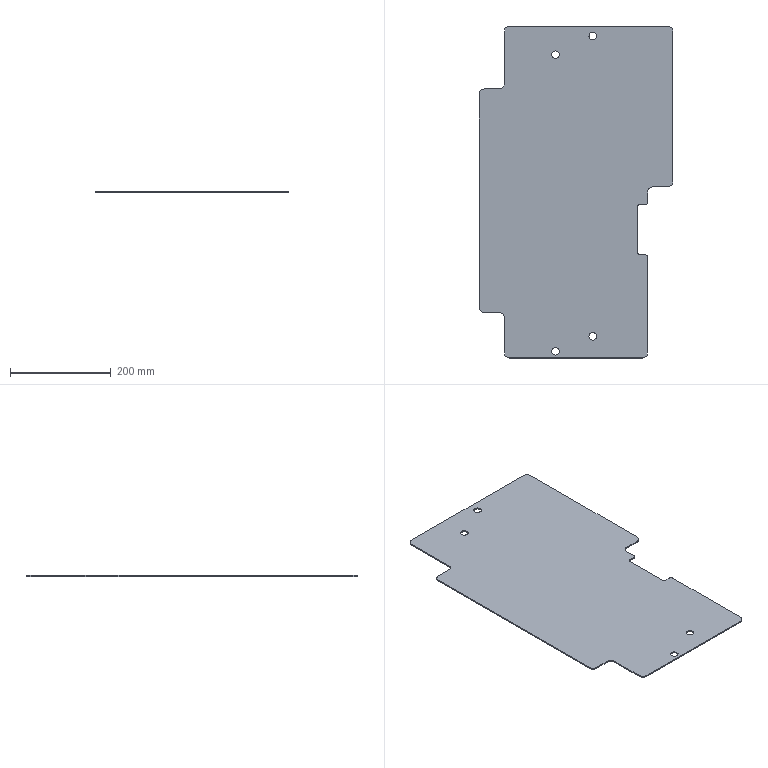Part | SolidWorks | features FlatPattern 1, SMBaseFlange 1, SheetMetal 1 | 1 solid | 38 faces | box 384.5 x 660 x 2.3 mm | volume 513423 mm3 | cylinder 22 | plane 16 | commonest cylinder face diameters 20 x10 15 x8 10 x4
STEP:
#1=CARTESIAN_POINT('',(163.,-881.,2.3));
#2=VERTEX_POINT('',#1);
#3=CARTESIAN_POINT('',(178.,-881.,2.3));
#4=VERTEX_POINT('',#3);
#5=CARTESIAN_POINT('',(170.5,-881.,2.3));
#6=DIRECTION('',(0.,0.,1.));
#7=DIRECTION('',(1.,0.,0.));
#8=AXIS2_PLACEMENT_3D('',#5,#6,#7);
#9=CIRCLE('',#8,7.5);
#10=EDGE_CURVE('',#2,#4,#9,.T.);
#11=ORIENTED_EDGE('',*,*,#10,.T.);
#12=CARTESIAN_POINT('',(178.,-881.,0.));
#13=VERTEX_POINT('',#12);
#14=CARTESIAN_POINT('',(178.,-881.,2.3));
#15=DIRECTION('',(0.,0.,-1.));
#16=VECTOR('',#15,1000.);
#17=LINE('',#14,#16);
#18=EDGE_CURVE('',#4,#13,#17,.T.);
#19=ORIENTED_EDGE('',*,*,#18,.T.);
#20=CARTESIAN_POINT('',(163.,-881.,0.));
#21=VERTEX_POINT('',#20);
#22=CARTESIAN_POINT('',(170.5,-881.,0.));
#23=DIRECTION('',(0.,0.,1.));
#24=DIRECTION('',(1.,0.,0.));
#25=AXIS2_PLACEMENT_3D('',#22,#23,#24);
#26=CIRCLE('',#25,7.5);
#27=EDGE_CURVE('',#21,#13,#26,.T.);
#28=ORIENTED_EDGE('',*,*,#27,.F.);
#29=CARTESIAN_POINT('',(163.,-881.,2.3));
#30=DIRECTION('',(0.,0.,-1.));
#31=VECTOR('',#30,1000.);
#32=LINE('',#29,#31);
#33=EDGE_CURVE('',#2,#21,#32,.T.);
#34=ORIENTED_EDGE('',*,*,#33,.F.);
#35=EDGE_LOOP('',(#11,#19,#28,#34));
#36=FACE_OUTER_BOUND('',#35,.T.);
#37=CARTESIAN_POINT('',(170.5,-881.,2.3));
#38=DIRECTION('',(0.,0.,-1.));
#39=DIRECTION('',(-1.,0.,0.));
#40=AXIS2_PLACEMENT_3D('',#37,#38,#39);
#41=CYLINDRICAL_SURFACE('',#40,7.5);
#42=ADVANCED_FACE('',(#36),#41,.F.);
#43=CARTESIAN_POINT('',(237.,-851.,2.3));
#44=VERTEX_POINT('',#43);
#45=CARTESIAN_POINT('',(252.,-851.,2.3));
#46=VERTEX_POINT('',#45);
#47=CARTESIAN_POINT('',(244.5,-851.,2.3));
#48=DIRECTION('',(0.,0.,1.));
#49=DIRECTION('',(1.,0.,0.));
#50=AXIS2_PLACEMENT_3D('',#47,#48,#49);
#51=CIRCLE('',#50,7.5);
#52=EDGE_CURVE('',#44,#46,#51,.T.);
#53=ORIENTED_EDGE('',*,*,#52,.T.);
#54=CARTESIAN_POINT('',(252.,-851.,0.));
#55=VERTEX_POINT('',#54);
#56=CARTESIAN_POINT('',(252.,-851.,2.3));
#57=DIRECTION('',(0.,0.,-1.));
#58=VECTOR('',#57,1000.);
#59=LINE('',#56,#58);
#60=EDGE_CURVE('',#46,#55,#59,.T.);
#61=ORIENTED_EDGE('',*,*,#60,.T.);
#62=CARTESIAN_POINT('',(237.,-851.,0.));
#63=VERTEX_POINT('',#62);
#64=CARTESIAN_POINT('',(244.5,-851.,0.));
#65=DIRECTION('',(0.,0.,1.));
#66=DIRECTION('',(1.,0.,0.));
#67=AXIS2_PLACEMENT_3D('',#64,#65,#66);
#68=CIRCLE('',#67,7.5);
#69=EDGE_CURVE('',#63,#55,#68,.T.);
#70=ORIENTED_EDGE('',*,*,#69,.F.);
#71=CARTESIAN_POINT('',(237.,-851.,2.3));
#72=DIRECTION('',(0.,0.,-1.));
#73=VECTOR('',#72,1000.);
#74=LINE('',#71,#73);
#75=EDGE_CURVE('',#44,#63,#74,.T.);
#76=ORIENTED_EDGE('',*,*,#75,.F.);
#77=EDGE_LOOP('',(#53,#61,#70,#76));
#78=FACE_OUTER_BOUND('',#77,.T.);
#79=CARTESIAN_POINT('',(244.5,-851.,2.3));
#80=DIRECTION('',(0.,0.,-1.));
#81=DIRECTION('',(-1.,0.,0.));
#82=AXIS2_PLACEMENT_3D('',#79,#80,#81);
#83=CYLINDRICAL_SURFACE('',#82,7.5);
#84=ADVANCED_FACE('',(#78),#83,.F.);
#85=CARTESIAN_POINT('',(237.,-254.,2.3));
#86=VERTEX_POINT('',#85);
#87=CARTESIAN_POINT('',(252.,-254.,2.3));
#88=VERTEX_POINT('',#87);
#89=CARTESIAN_POINT('',(244.5,-254.,2.3));
#90=DIRECTION('',(0.,0.,1.));
#91=DIRECTION('',(1.,0.,0.));
#92=AXIS2_PLACEMENT_3D('',#89,#90,#91);
#93=CIRCLE('',#92,7.5);
#94=EDGE_CURVE('',#86,#88,#93,.T.);
#95=ORIENTED_EDGE('',*,*,#94,.T.);
#96=CARTESIAN_POINT('',(252.,-254.,0.));
#97=VERTEX_POINT('',#96);
#98=CARTESIAN_POINT('',(252.,-254.,2.3));
#99=DIRECTION('',(0.,0.,-1.));
#100=VECTOR('',#99,1000.);
#101=LINE('',#98,#100);
#102=EDGE_CURVE('',#88,#97,#101,.T.);
#103=ORIENTED_EDGE('',*,*,#102,.T.);
#104=CARTESIAN_POINT('',(237.,-254.,0.));
#105=VERTEX_POINT('',#104);
#106=CARTESIAN_POINT('',(244.5,-254.,0.));
#107=DIRECTION('',(0.,0.,1.));
#108=DIRECTION('',(1.,0.,0.));
#109=AXIS2_PLACEMENT_3D('',#106,#107,#108);
#110=CIRCLE('',#109,7.5);
#111=EDGE_CURVE('',#105,#97,#110,.T.);
#112=ORIENTED_EDGE('',*,*,#111,.F.);
#113=CARTESIAN_POINT('',(237.,-254.,2.3));
#114=DIRECTION('',(0.,0.,-1.));
#115=VECTOR('',#114,1000.);
#116=LINE('',#113,#115);
#117=EDGE_CURVE('',#86,#105,#116,.T.);
#118=ORIENTED_EDGE('',*,*,#117,.F.);
#119=EDGE_LOOP('',(#95,#103,#112,#118));
#120=FACE_OUTER_BOUND('',#119,.T.);
#121=CARTESIAN_POINT('',(244.5,-254.,2.3));
#122=DIRECTION('',(0.,0.,-1.));
#123=DIRECTION('',(-1.,0.,0.));
#124=AXIS2_PLACEMENT_3D('',#121,#122,#123);
#125=CYLINDRICAL_SURFACE('',#124,7.5);
#126=ADVANCED_FACE('',(#120),#125,.F.);
#127=CARTESIAN_POINT('',(163.,-291.,2.3));
#128=VERTEX_POINT('',#127);
#129=CARTESIAN_POINT('',(178.,-291.,2.3));
#130=VERTEX_POINT('',#129);
#131=CARTESIAN_POINT('',(170.5,-291.,2.3));
#132=DIRECTION('',(0.,0.,1.));
#133=DIRECTION('',(1.,0.,0.));
#134=AXIS2_PLACEMENT_3D('',#131,#132,#133);
#135=CIRCLE('',#134,7.5);
#136=EDGE_CURVE('',#128,#130,#135,.T.);
#137=ORIENTED_EDGE('',*,*,#136,.T.);
#138=CARTESIAN_POINT('',(178.,-291.,0.));
#139=VERTEX_POINT('',#138);
#140=CARTESIAN_POINT('',(178.,-291.,2.3));
#141=DIRECTION('',(0.,0.,-1.));
#142=VECTOR('',#141,1000.);
#143=LINE('',#140,#142);
#144=EDGE_CURVE('',#130,#139,#143,.T.);
#145=ORIENTED_EDGE('',*,*,#144,.T.);
#146=CARTESIAN_POINT('',(163.,-291.,0.));
#147=VERTEX_POINT('',#146);
#148=CARTESIAN_POINT('',(170.5,-291.,0.));
#149=DIRECTION('',(0.,0.,1.));
#150=DIRECTION('',(1.,0.,0.));
#151=AXIS2_PLACEMENT_3D('',#148,#149,#150);
#152=CIRCLE('',#151,7.5);
#153=EDGE_CURVE('',#147,#139,#152,.T.);
#154=ORIENTED_EDGE('',*,*,#153,.F.);
#155=CARTESIAN_POINT('',(163.,-291.,2.3));
#156=DIRECTION('',(0.,0.,-1.));
#157=VECTOR('',#156,1000.);
#158=LINE('',#155,#157);
#159=EDGE_CURVE('',#128,#147,#158,.T.);
#160=ORIENTED_EDGE('',*,*,#159,.F.);
#161=EDGE_LOOP('',(#137,#145,#154,#160));
#162=FACE_OUTER_BOUND('',#161,.T.);
#163=CARTESIAN_POINT('',(170.5,-291.,2.3));
#164=DIRECTION('',(0.,0.,-1.));
#165=DIRECTION('',(-1.,0.,0.));
#166=AXIS2_PLACEMENT_3D('',#163,#164,#165);
#167=CYLINDRICAL_SURFACE('',#166,7.5);
#168=ADVANCED_FACE('',(#162),#167,.F.);
#169=CARTESIAN_POINT('',(29.,-359.,2.3));
#170=VERTEX_POINT('',#169);
#171=CARTESIAN_POINT('',(19.,-369.,2.3));
#172=VERTEX_POINT('',#171);
#173=CARTESIAN_POINT('',(29.,-369.,2.3));
#174=DIRECTION('',(0.,0.,1.));
#175=DIRECTION('',(-1.,0.,0.));
#176=AXIS2_PLACEMENT_3D('',#173,#174,#175);
#177=CIRCLE('',#176,10.);
#178=EDGE_CURVE('',#170,#172,#177,.T.);
#179=ORIENTED_EDGE('',*,*,#178,.T.);
#180=CARTESIAN_POINT('',(19.,-794.,2.3));
#181=VERTEX_POINT('',#180);
#182=CARTESIAN_POINT('',(19.,-794.,2.3));
#183=DIRECTION('',(0.,-1.,0.));
#184=VECTOR('',#183,1000.);
#185=LINE('',#182,#184);
#186=EDGE_CURVE('',#172,#181,#185,.T.);
#187=ORIENTED_EDGE('',*,*,#186,.T.);
#188=CARTESIAN_POINT('',(29.,-804.,2.3));
#189=VERTEX_POINT('',#188);
#190=CARTESIAN_POINT('',(29.,-794.,2.3));
#191=DIRECTION('',(0.,0.,1.));
#192=DIRECTION('',(-1.,0.,0.));
#193=AXIS2_PLACEMENT_3D('',#190,#191,#192);
#194=CIRCLE('',#193,10.);
#195=EDGE_CURVE('',#181,#189,#194,.T.);
#196=ORIENTED_EDGE('',*,*,#195,.T.);
#197=CARTESIAN_POINT('',(59.,-804.,2.3));
#198=VERTEX_POINT('',#197);
#199=CARTESIAN_POINT('',(59.,-804.,2.3));
#200=DIRECTION('',(1.,0.,0.));
#201=VECTOR('',#200,1000.);
#202=LINE('',#199,#201);
#203=EDGE_CURVE('',#189,#198,#202,.T.);
#204=ORIENTED_EDGE('',*,*,#203,.T.);
#205=CARTESIAN_POINT('',(69.,-814.,2.3));
#206=VERTEX_POINT('',#205);
#207=CARTESIAN_POINT('',(59.,-814.,2.3));
#208=DIRECTION('',(0.,0.,-1.));
#209=DIRECTION('',(1.,0.,0.));
#210=AXIS2_PLACEMENT_3D('',#207,#208,#209);
#211=CIRCLE('',#210,10.);
#212=EDGE_CURVE('',#198,#206,#211,.T.);
#213=ORIENTED_EDGE('',*,*,#212,.T.);
#214=CARTESIAN_POINT('',(69.,-884.,2.3));
#215=VERTEX_POINT('',#214);
#216=CARTESIAN_POINT('',(69.,-884.,2.3));
#217=DIRECTION('',(0.,-1.,0.));
#218=VECTOR('',#217,1000.);
#219=LINE('',#216,#218);
#220=EDGE_CURVE('',#206,#215,#219,.T.);
#221=ORIENTED_EDGE('',*,*,#220,.T.);
#222=CARTESIAN_POINT('',(79.,-894.,2.3));
#223=VERTEX_POINT('',#222);
#224=CARTESIAN_POINT('',(79.,-884.,2.3));
#225=DIRECTION('',(0.,0.,1.));
#226=DIRECTION('',(-1.,0.,0.));
#227=AXIS2_PLACEMENT_3D('',#224,#225,#226);
#228=CIRCLE('',#227,10.);
#229=EDGE_CURVE('',#215,#223,#228,.T.);
#230=ORIENTED_EDGE('',*,*,#229,.T.);
#231=CARTESIAN_POINT('',(343.5,-894.,2.3));
#232=VERTEX_POINT('',#231);
#233=CARTESIAN_POINT('',(343.5,-894.,2.3));
#234=DIRECTION('',(1.,0.,0.));
#235=VECTOR('',#234,1000.);
#236=LINE('',#233,#235);
#237=EDGE_CURVE('',#223,#232,#236,.T.);
#238=ORIENTED_EDGE('',*,*,#237,.T.);
#239=CARTESIAN_POINT('',(353.5,-884.,2.3));
#240=VERTEX_POINT('',#239);
#241=CARTESIAN_POINT('',(343.5,-884.,2.3));
#242=DIRECTION('',(0.,0.,1.));
#243=DIRECTION('',(-1.,0.,0.));
#244=AXIS2_PLACEMENT_3D('',#241,#242,#243);
#245=CIRCLE('',#244,10.);
#246=EDGE_CURVE('',#232,#240,#245,.T.);
#247=ORIENTED_EDGE('',*,*,#246,.T.);
#248=CARTESIAN_POINT('',(353.5,-694.,2.3));
#249=VERTEX_POINT('',#248);
#250=CARTESIAN_POINT('',(353.5,-694.,2.3));
#251=DIRECTION('',(0.,1.,0.));
#252=VECTOR('',#251,1000.);
#253=LINE('',#250,#252);
#254=EDGE_CURVE('',#240,#249,#253,.T.);
#255=ORIENTED_EDGE('',*,*,#254,.T.);
#256=CARTESIAN_POINT('',(348.5,-689.,2.3));
#257=VERTEX_POINT('',#256);
#258=CARTESIAN_POINT('',(348.5,-694.,2.3));
#259=DIRECTION('',(0.,0.,1.));
#260=DIRECTION('',(-1.,0.,0.));
#261=AXIS2_PLACEMENT_3D('',#258,#259,#260);
#262=CIRCLE('',#261,5.);
#263=EDGE_CURVE('',#249,#257,#262,.T.);
#264=ORIENTED_EDGE('',*,*,#263,.T.);
#265=CARTESIAN_POINT('',(338.5,-689.,2.3));
#266=VERTEX_POINT('',#265);
#267=CARTESIAN_POINT('',(338.5,-689.,2.3));
#268=DIRECTION('',(-1.,0.,0.));
#269=VECTOR('',#268,1000.);
#270=LINE('',#267,#269);
#271=EDGE_CURVE('',#257,#266,#270,.T.);
#272=ORIENTED_EDGE('',*,*,#271,.T.);
#273=CARTESIAN_POINT('',(333.5,-684.,2.3));
#274=VERTEX_POINT('',#273);
#275=CARTESIAN_POINT('',(338.5,-684.,2.3));
#276=DIRECTION('',(0.,0.,-1.));
#277=DIRECTION('',(1.,0.,0.));
#278=AXIS2_PLACEMENT_3D('',#275,#276,#277);
#279=CIRCLE('',#278,5.);
#280=EDGE_CURVE('',#266,#274,#279,.T.);
#281=ORIENTED_EDGE('',*,*,#280,.T.);
#282=CARTESIAN_POINT('',(333.5,-594.,2.3));
#283=VERTEX_POINT('',#282);
#284=CARTESIAN_POINT('',(333.5,-594.,2.3));
#285=DIRECTION('',(0.,1.,0.));
#286=VECTOR('',#285,1000.);
#287=LINE('',#284,#286);
#288=EDGE_CURVE('',#274,#283,#287,.T.);
#289=ORIENTED_EDGE('',*,*,#288,.T.);
#290=CARTESIAN_POINT('',(338.5,-589.,2.3));
#291=VERTEX_POINT('',#290);
#292=CARTESIAN_POINT('',(338.5,-594.,2.3));
#293=DIRECTION('',(0.,0.,-1.));
#294=DIRECTION('',(1.,0.,0.));
#295=AXIS2_PLACEMENT_3D('',#292,#293,#294);
#296=CIRCLE('',#295,5.);
#297=EDGE_CURVE('',#283,#291,#296,.T.);
#298=ORIENTED_EDGE('',*,*,#297,.T.);
#299=CARTESIAN_POINT('',(348.5,-589.,2.3));
#300=VERTEX_POINT('',#299);
#301=CARTESIAN_POINT('',(348.5,-589.,2.3));
#302=DIRECTION('',(1.,0.,0.));
#303=VECTOR('',#302,1000.);
#304=LINE('',#301,#303);
#305=EDGE_CURVE('',#291,#300,#304,.T.);
#306=ORIENTED_EDGE('',*,*,#305,.T.);
#307=CARTESIAN_POINT('',(353.5,-584.,2.3));
#308=VERTEX_POINT('',#307);
#309=CARTESIAN_POINT('',(348.5,-584.,2.3));
#310=DIRECTION('',(0.,0.,1.));
#311=DIRECTION('',(1.,0.,0.));
#312=AXIS2_PLACEMENT_3D('',#309,#310,#311);
#313=CIRCLE('',#312,5.);
#314=EDGE_CURVE('',#300,#308,#313,.T.);
#315=ORIENTED_EDGE('',*,*,#314,.T.);
#316=CARTESIAN_POINT('',(353.5,-564.,2.3));
#317=VERTEX_POINT('',#316);
#318=CARTESIAN_POINT('',(353.5,-564.,2.3));
#319=DIRECTION('',(0.,1.,0.));
#320=VECTOR('',#319,1000.);
#321=LINE('',#318,#320);
#322=EDGE_CURVE('',#308,#317,#321,.T.);
#323=ORIENTED_EDGE('',*,*,#322,.T.);
#324=CARTESIAN_POINT('',(363.5,-554.,2.3));
#325=VERTEX_POINT('',#324);
#326=CARTESIAN_POINT('',(363.5,-564.,2.3));
#327=DIRECTION('',(0.,0.,-1.));
#328=DIRECTION('',(1.,0.,0.));
#329=AXIS2_PLACEMENT_3D('',#326,#327,#328);
#330=CIRCLE('',#329,10.);
#331=EDGE_CURVE('',#317,#325,#330,.T.);
#332=ORIENTED_EDGE('',*,*,#331,.T.);
#333=CARTESIAN_POINT('',(393.5,-554.,2.3));
#334=VERTEX_POINT('',#333);
#335=CARTESIAN_POINT('',(393.5,-554.,2.3));
#336=DIRECTION('',(1.,0.,0.));
#337=VECTOR('',#336,1000.);
#338=LINE('',#335,#337);
#339=EDGE_CURVE('',#325,#334,#338,.T.);
#340=ORIENTED_EDGE('',*,*,#339,.T.);
#341=CARTESIAN_POINT('',(403.5,-544.,2.3));
#342=VERTEX_POINT('',#341);
#343=CARTESIAN_POINT('',(393.5,-544.,2.3));
#344=DIRECTION('',(0.,0.,1.));
#345=DIRECTION('',(-1.,0.,0.));
#346=AXIS2_PLACEMENT_3D('',#343,#344,#345);
#347=CIRCLE('',#346,10.);
#348=EDGE_CURVE('',#334,#342,#347,.T.);
#349=ORIENTED_EDGE('',*,*,#348,.T.);
#350=CARTESIAN_POINT('',(403.5,-244.,2.3));
#351=VERTEX_POINT('',#350);
#352=CARTESIAN_POINT('',(403.5,-244.,2.3));
#353=DIRECTION('',(0.,1.,0.));
#354=VECTOR('',#353,1000.);
#355=LINE('',#352,#354);
#356=EDGE_CURVE('',#342,#351,#355,.T.);
#357=ORIENTED_EDGE('',*,*,#356,.T.);
#358=CARTESIAN_POINT('',(393.5,-234.,2.3));
#359=VERTEX_POINT('',#358);
#360=CARTESIAN_POINT('',(393.5,-244.,2.3));
#361=DIRECTION('',(0.,0.,1.));
#362=DIRECTION('',(-1.,0.,0.));
#363=AXIS2_PLACEMENT_3D('',#360,#361,#362);
#364=CIRCLE('',#363,10.);
#365=EDGE_CURVE('',#351,#359,#364,.T.);
#366=ORIENTED_EDGE('',*,*,#365,.T.);
#367=CARTESIAN_POINT('',(79.,-234.,2.3));
#368=VERTEX_POINT('',#367);
#369=CARTESIAN_POINT('',(79.,-234.,2.3));
#370=DIRECTION('',(-1.,0.,0.));
#371=VECTOR('',#370,1000.);
#372=LINE('',#369,#371);
#373=EDGE_CURVE('',#359,#368,#372,.T.);
#374=ORIENTED_EDGE('',*,*,#373,.T.);
#375=CARTESIAN_POINT('',(69.,-244.,2.3));
#376=VERTEX_POINT('',#375);
#377=CARTESIAN_POINT('',(79.,-244.,2.3));
#378=DIRECTION('',(0.,0.,1.));
#379=DIRECTION('',(-1.,0.,0.));
#380=AXIS2_PLACEMENT_3D('',#377,#378,#379);
#381=CIRCLE('',#380,10.);
#382=EDGE_CURVE('',#368,#376,#381,.T.);
#383=ORIENTED_EDGE('',*,*,#382,.T.);
#384=CARTESIAN_POINT('',(69.,-349.,2.3));
#385=VERTEX_POINT('',#384);
#386=CARTESIAN_POINT('',(69.,-349.,2.3));
#387=DIRECTION('',(0.,-1.,0.));
#388=VECTOR('',#387,1000.);
#389=LINE('',#386,#388);
#390=EDGE_CURVE('',#376,#385,#389,.T.);
#391=ORIENTED_EDGE('',*,*,#390,.T.);
#392=CARTESIAN_POINT('',(59.,-359.,2.3));
#393=VERTEX_POINT('',#392);
#394=CARTESIAN_POINT('',(59.,-349.,2.3));
#395=DIRECTION('',(0.,0.,-1.));
#396=DIRECTION('',(1.,0.,0.));
#397=AXIS2_PLACEMENT_3D('',#394,#395,#396);
#398=CIRCLE('',#397,10.);
#399=EDGE_CURVE('',#385,#393,#398,.T.);
#400=ORIENTED_EDGE('',*,*,#399,.T.);
#401=CARTESIAN_POINT('',(29.,-359.,2.3));
#402=DIRECTION('',(-1.,0.,0.));
#403=VECTOR('',#402,1000.);
#404=LINE('',#401,#403);
#405=EDGE_CURVE('',#393,#170,#404,.T.);
#406=ORIENTED_EDGE('',*,*,#405,.T.);
#407=EDGE_LOOP('',(#179,#187,#196,#204,#213,#221,#230,#238,#247,#255,#264,#272,#281,#289,#298,#306,#315,#323,#332,#340,#349,#357,#366,#374,#383,#391,#400,#406));
#408=FACE_OUTER_BOUND('',#407,.T.);
#409=ORIENTED_EDGE('',*,*,#136,.F.);
#410=CARTESIAN_POINT('',(170.5,-291.,2.3));
#411=DIRECTION('',(0.,0.,1.));
#412=DIRECTION('',(1.,0.,0.));
#413=AXIS2_PLACEMENT_3D('',#410,#411,#412);
#414=CIRCLE('',#413,7.5);
#415=EDGE_CURVE('',#130,#128,#414,.T.);
#416=ORIENTED_EDGE('',*,*,#415,.F.);
#417=EDGE_LOOP('',(#409,#416));
#418=FACE_BOUND('',#417,.T.);
#419=ORIENTED_EDGE('',*,*,#94,.F.);
#420=CARTESIAN_POINT('',(244.5,-254.,2.3));
#421=DIRECTION('',(0.,0.,1.));
#422=DIRECTION('',(1.,0.,0.));
#423=AXIS2_PLACEMENT_3D('',#420,#421,#422);
#424=CIRCLE('',#423,7.5);
#425=EDGE_CURVE('',#88,#86,#424,.T.);
#426=ORIENTED_EDGE('',*,*,#425,.F.);
#427=EDGE_LOOP('',(#419,#426));
#428=FACE_BOUND('',#427,.T.);
#429=ORIENTED_EDGE('',*,*,#52,.F.);
#430=CARTESIAN_POINT('',(244.5,-851.,2.3));
#431=DIRECTION('',(0.,0.,1.));
#432=DIRECTION('',(1.,0.,0.));
#433=AXIS2_PLACEMENT_3D('',#430,#431,#432);
#434=CIRCLE('',#433,7.5);
#435=EDGE_CURVE('',#46,#44,#434,.T.);
#436=ORIENTED_EDGE('',*,*,#435,.F.);
#437=EDGE_LOOP('',(#429,#436));
#438=FACE_BOUND('',#437,.T.);
#439=ORIENTED_EDGE('',*,*,#10,.F.);
#440=CARTESIAN_POINT('',(170.5,-881.,2.3));
#441=DIRECTION('',(0.,0.,1.));
#442=DIRECTION('',(1.,0.,0.));
#443=AXIS2_PLACEMENT_3D('',#440,#441,#442);
#444=CIRCLE('',#443,7.5);
#445=EDGE_CURVE('',#4,#2,#444,.T.);
#446=ORIENTED_EDGE('',*,*,#445,.F.);
#447=EDGE_LOOP('',(#439,#446));
#448=FACE_BOUND('',#447,.T.);
#449=CARTESIAN_POINT('',(29.,-369.,2.3));
#450=DIRECTION('',(0.,0.,-1.));
#451=DIRECTION('',(-1.,0.,0.));
#452=AXIS2_PLACEMENT_3D('',#449,#450,#451);
#453=PLANE('',#452);
#454=ADVANCED_FACE('',(#408,#418,#428,#438,#448),#453,.F.);
#455=ORIENTED_EDGE('',*,*,#69,.T.);
#456=CARTESIAN_POINT('',(244.5,-851.,0.));
#457=DIRECTION('',(0.,0.,1.));
#458=DIRECTION('',(1.,0.,0.));
#459=AXIS2_PLACEMENT_3D('',#456,#457,#458);
#460=CIRCLE('',#459,7.5);
#461=EDGE_CURVE('',#55,#63,#460,.T.);
#462=ORIENTED_EDGE('',*,*,#461,.T.);
#463=EDGE_LOOP('',(#455,#462));
#464=FACE_BOUND('',#463,.T.);
#465=ORIENTED_EDGE('',*,*,#153,.T.);
#466=CARTESIAN_POINT('',(170.5,-291.,0.));
#467=DIRECTION('',(0.,0.,1.));
#468=DIRECTION('',(1.,0.,0.));
#469=AXIS2_PLACEMENT_3D('',#466,#467,#468);
#470=CIRCLE('',#469,7.5);
#471=EDGE_CURVE('',#139,#147,#470,.T.);
#472=ORIENTED_EDGE('',*,*,#471,.T.);
#473=EDGE_LOOP('',(#465,#472));
#474=FACE_BOUND('',#473,.T.);
#475=CARTESIAN_POINT('',(29.,-359.,0.));
#476=VERTEX_POINT('',#475);
#477=CARTESIAN_POINT('',(19.,-369.,0.));
#478=VERTEX_POINT('',#477);
#479=CARTESIAN_POINT('',(29.,-369.,0.));
#480=DIRECTION('',(0.,0.,1.));
#481=DIRECTION('',(-1.,0.,0.));
#482=AXIS2_PLACEMENT_3D('',#479,#480,#481);
#483=CIRCLE('',#482,10.);
#484=EDGE_CURVE('',#476,#478,#483,.T.);
#485=ORIENTED_EDGE('',*,*,#484,.F.);
#486=CARTESIAN_POINT('',(59.,-359.,0.));
#487=VERTEX_POINT('',#486);
#488=CARTESIAN_POINT('',(29.,-359.,0.));
#489=DIRECTION('',(-1.,0.,0.));
#490=VECTOR('',#489,1000.);
#491=LINE('',#488,#490);
#492=EDGE_CURVE('',#487,#476,#491,.T.);
#493=ORIENTED_EDGE('',*,*,#492,.F.);
#494=CARTESIAN_POINT('',(69.,-349.,0.));
#495=VERTEX_POINT('',#494);
#496=CARTESIAN_POINT('',(59.,-349.,0.));
#497=DIRECTION('',(0.,0.,-1.));
#498=DIRECTION('',(1.,0.,0.));
#499=AXIS2_PLACEMENT_3D('',#496,#497,#498);
#500=CIRCLE('',#499,10.);
#501=EDGE_CURVE('',#495,#487,#500,.T.);
#502=ORIENTED_EDGE('',*,*,#501,.F.);
#503=CARTESIAN_POINT('',(69.,-244.,0.));
#504=VERTEX_POINT('',#503);
#505=CARTESIAN_POINT('',(69.,-349.,0.));
#506=DIRECTION('',(0.,-1.,0.));
#507=VECTOR('',#506,1000.);
#508=LINE('',#505,#507);
#509=EDGE_CURVE('',#504,#495,#508,.T.);
#510=ORIENTED_EDGE('',*,*,#509,.F.);
#511=CARTESIAN_POINT('',(79.,-234.,0.));
#512=VERTEX_POINT('',#511);
#513=CARTESIAN_POINT('',(79.,-244.,0.));
#514=DIRECTION('',(0.,0.,1.));
#515=DIRECTION('',(-1.,0.,0.));
#516=AXIS2_PLACEMENT_3D('',#513,#514,#515);
#517=CIRCLE('',#516,10.);
#518=EDGE_CURVE('',#512,#504,#517,.T.);
#519=ORIENTED_EDGE('',*,*,#518,.F.);
#520=CARTESIAN_POINT('',(393.5,-234.,0.));
#521=VERTEX_POINT('',#520);
#522=CARTESIAN_POINT('',(79.,-234.,0.));
#523=DIRECTION('',(-1.,0.,0.));
#524=VECTOR('',#523,1000.);
#525=LINE('',#522,#524);
#526=EDGE_CURVE('',#521,#512,#525,.T.);
#527=ORIENTED_EDGE('',*,*,#526,.F.);
#528=CARTESIAN_POINT('',(403.5,-244.,0.));
#529=VERTEX_POINT('',#528);
#530=CARTESIAN_POINT('',(393.5,-244.,0.));
#531=DIRECTION('',(0.,0.,1.));
#532=DIRECTION('',(-1.,0.,0.));
#533=AXIS2_PLACEMENT_3D('',#530,#531,#532);
#534=CIRCLE('',#533,10.);
#535=EDGE_CURVE('',#529,#521,#534,.T.);
#536=ORIENTED_EDGE('',*,*,#535,.F.);
#537=CARTESIAN_POINT('',(403.5,-544.,0.));
#538=VERTEX_POINT('',#537);
#539=CARTESIAN_POINT('',(403.5,-244.,0.));
#540=DIRECTION('',(0.,1.,0.));
#541=VECTOR('',#540,1000.);
#542=LINE('',#539,#541);
#543=EDGE_CURVE('',#538,#529,#542,.T.);
#544=ORIENTED_EDGE('',*,*,#543,.F.);
#545=CARTESIAN_POINT('',(393.5,-554.,0.));
#546=VERTEX_POINT('',#545);
#547=CARTESIAN_POINT('',(393.5,-544.,0.));
#548=DIRECTION('',(0.,0.,1.));
#549=DIRECTION('',(-1.,0.,0.));
#550=AXIS2_PLACEMENT_3D('',#547,#548,#549);
#551=CIRCLE('',#550,10.);
#552=EDGE_CURVE('',#546,#538,#551,.T.);
#553=ORIENTED_EDGE('',*,*,#552,.F.);
#554=CARTESIAN_POINT('',(363.5,-554.,0.));
#555=VERTEX_POINT('',#554);
#556=CARTESIAN_POINT('',(393.5,-554.,0.));
#557=DIRECTION('',(1.,0.,0.));
#558=VECTOR('',#557,1000.);
#559=LINE('',#556,#558);
#560=EDGE_CURVE('',#555,#546,#559,.T.);
#561=ORIENTED_EDGE('',*,*,#560,.F.);
#562=CARTESIAN_POINT('',(353.5,-564.,0.));
#563=VERTEX_POINT('',#562);
#564=CARTESIAN_POINT('',(363.5,-564.,0.));
#565=DIRECTION('',(0.,0.,-1.));
#566=DIRECTION('',(1.,0.,0.));
#567=AXIS2_PLACEMENT_3D('',#564,#565,#566);
#568=CIRCLE('',#567,10.);
#569=EDGE_CURVE('',#563,#555,#568,.T.);
#570=ORIENTED_EDGE('',*,*,#569,.F.);
#571=CARTESIAN_POINT('',(353.5,-584.,0.));
#572=VERTEX_POINT('',#571);
#573=CARTESIAN_POINT('',(353.5,-564.,0.));
#574=DIRECTION('',(0.,1.,0.));
#575=VECTOR('',#574,1000.);
#576=LINE('',#573,#575);
#577=EDGE_CURVE('',#572,#563,#576,.T.);
#578=ORIENTED_EDGE('',*,*,#577,.F.);
#579=CARTESIAN_POINT('',(348.5,-589.,0.));
#580=VERTEX_POINT('',#579);
#581=CARTESIAN_POINT('',(348.5,-584.,0.));
#582=DIRECTION('',(0.,0.,1.));
#583=DIRECTION('',(1.,0.,0.));
#584=AXIS2_PLACEMENT_3D('',#581,#582,#583);
#585=CIRCLE('',#584,5.);
#586=EDGE_CURVE('',#580,#572,#585,.T.);
#587=ORIENTED_EDGE('',*,*,#586,.F.);
#588=CARTESIAN_POINT('',(338.5,-589.,0.));
#589=VERTEX_POINT('',#588);
#590=CARTESIAN_POINT('',(348.5,-589.,0.));
#591=DIRECTION('',(1.,0.,0.));
#592=VECTOR('',#591,1000.);
#593=LINE('',#590,#592);
#594=EDGE_CURVE('',#589,#580,#593,.T.);
#595=ORIENTED_EDGE('',*,*,#594,.F.);
#596=CARTESIAN_POINT('',(333.5,-594.,0.));
#597=VERTEX_POINT('',#596);
#598=CARTESIAN_POINT('',(338.5,-594.,0.));
#599=DIRECTION('',(0.,0.,-1.));
#600=DIRECTION('',(1.,0.,0.));
#601=AXIS2_PLACEMENT_3D('',#598,#599,#600);
#602=CIRCLE('',#601,5.);
#603=EDGE_CURVE('',#597,#589,#602,.T.);
#604=ORIENTED_EDGE('',*,*,#603,.F.);
#605=CARTESIAN_POINT('',(333.5,-684.,0.));
#606=VERTEX_POINT('',#605);
#607=CARTESIAN_POINT('',(333.5,-594.,0.));
#608=DIRECTION('',(0.,1.,0.));
#609=VECTOR('',#608,1000.);
#610=LINE('',#607,#609);
#611=EDGE_CURVE('',#606,#597,#610,.T.);
#612=ORIENTED_EDGE('',*,*,#611,.F.);
#613=CARTESIAN_POINT('',(338.5,-689.,0.));
#614=VERTEX_POINT('',#613);
#615=CARTESIAN_POINT('',(338.5,-684.,0.));
#616=DIRECTION('',(0.,0.,-1.));
#617=DIRECTION('',(1.,0.,0.));
#618=AXIS2_PLACEMENT_3D('',#615,#616,#617);
#619=CIRCLE('',#618,5.);
#620=EDGE_CURVE('',#614,#606,#619,.T.);
#621=ORIENTED_EDGE('',*,*,#620,.F.);
#622=CARTESIAN_POINT('',(348.5,-689.,0.));
#623=VERTEX_POINT('',#622);
#624=CARTESIAN_POINT('',(338.5,-689.,0.));
#625=DIRECTION('',(-1.,0.,0.));
#626=VECTOR('',#625,1000.);
#627=LINE('',#624,#626);
#628=EDGE_CURVE('',#623,#614,#627,.T.);
#629=ORIENTED_EDGE('',*,*,#628,.F.);
#630=CARTESIAN_POINT('',(353.5,-694.,0.));
#631=VERTEX_POINT('',#630);
#632=CARTESIAN_POINT('',(348.5,-694.,0.));
#633=DIRECTION('',(0.,0.,1.));
#634=DIRECTION('',(-1.,0.,0.));
#635=AXIS2_PLACEMENT_3D('',#632,#633,#634);
#636=CIRCLE('',#635,5.);
#637=EDGE_CURVE('',#631,#623,#636,.T.);
#638=ORIENTED_EDGE('',*,*,#637,.F.);
#639=CARTESIAN_POINT('',(353.5,-884.,0.));
#640=VERTEX_POINT('',#639);
#641=CARTESIAN_POINT('',(353.5,-694.,0.));
#642=DIRECTION('',(0.,1.,0.));
#643=VECTOR('',#642,1000.);
#644=LINE('',#641,#643);
#645=EDGE_CURVE('',#640,#631,#644,.T.);
#646=ORIENTED_EDGE('',*,*,#645,.F.);
#647=CARTESIAN_POINT('',(343.5,-894.,0.));
#648=VERTEX_POINT('',#647);
#649=CARTESIAN_POINT('',(343.5,-884.,0.));
#650=DIRECTION('',(0.,0.,1.));
#651=DIRECTION('',(-1.,0.,0.));
#652=AXIS2_PLACEMENT_3D('',#649,#650,#651);
#653=CIRCLE('',#652,10.);
#654=EDGE_CURVE('',#648,#640,#653,.T.);
#655=ORIENTED_EDGE('',*,*,#654,.F.);
#656=CARTESIAN_POINT('',(79.,-894.,0.));
#657=VERTEX_POINT('',#656);
#658=CARTESIAN_POINT('',(343.5,-894.,0.));
#659=DIRECTION('',(1.,0.,0.));
#660=VECTOR('',#659,1000.);
#661=LINE('',#658,#660);
#662=EDGE_CURVE('',#657,#648,#661,.T.);
#663=ORIENTED_EDGE('',*,*,#662,.F.);
#664=CARTESIAN_POINT('',(69.,-884.,0.));
#665=VERTEX_POINT('',#664);
#666=CARTESIAN_POINT('',(79.,-884.,0.));
#667=DIRECTION('',(0.,0.,1.));
#668=DIRECTION('',(-1.,0.,0.));
#669=AXIS2_PLACEMENT_3D('',#666,#667,#668);
#670=CIRCLE('',#669,10.);
#671=EDGE_CURVE('',#665,#657,#670,.T.);
#672=ORIENTED_EDGE('',*,*,#671,.F.);
#673=CARTESIAN_POINT('',(69.,-814.,0.));
#674=VERTEX_POINT('',#673);
#675=CARTESIAN_POINT('',(69.,-884.,0.));
#676=DIRECTION('',(0.,-1.,0.));
#677=VECTOR('',#676,1000.);
#678=LINE('',#675,#677);
#679=EDGE_CURVE('',#674,#665,#678,.T.);
#680=ORIENTED_EDGE('',*,*,#679,.F.);
#681=CARTESIAN_POINT('',(59.,-804.,0.));
#682=VERTEX_POINT('',#681);
#683=CARTESIAN_POINT('',(59.,-814.,0.));
#684=DIRECTION('',(0.,0.,-1.));
#685=DIRECTION('',(1.,0.,0.));
#686=AXIS2_PLACEMENT_3D('',#683,#684,#685);
#687=CIRCLE('',#686,10.);
#688=EDGE_CURVE('',#682,#674,#687,.T.);
#689=ORIENTED_EDGE('',*,*,#688,.F.);
#690=CARTESIAN_POINT('',(29.,-804.,0.));
#691=VERTEX_POINT('',#690);
#692=CARTESIAN_POINT('',(59.,-804.,0.));
#693=DIRECTION('',(1.,0.,0.));
#694=VECTOR('',#693,1000.);
#695=LINE('',#692,#694);
#696=EDGE_CURVE('',#691,#682,#695,.T.);
#697=ORIENTED_EDGE('',*,*,#696,.F.);
#698=CARTESIAN_POINT('',(19.,-794.,0.));
#699=VERTEX_POINT('',#698);
#700=CARTESIAN_POINT('',(29.,-794.,0.));
#701=DIRECTION('',(0.,0.,1.));
#702=DIRECTION('',(-1.,0.,0.));
#703=AXIS2_PLACEMENT_3D('',#700,#701,#702);
#704=CIRCLE('',#703,10.);
#705=EDGE_CURVE('',#699,#691,#704,.T.);
#706=ORIENTED_EDGE('',*,*,#705,.F.);
#707=CARTESIAN_POINT('',(19.,-794.,0.));
#708=DIRECTION('',(0.,-1.,0.));
#709=VECTOR('',#708,1000.);
#710=LINE('',#707,#709);
#711=EDGE_CURVE('',#478,#699,#710,.T.);
#712=ORIENTED_EDGE('',*,*,#711,.F.);
#713=EDGE_LOOP('',(#485,#493,#502,#510,#519,#527,#536,#544,#553,#561,#570,#578,#587,#595,#604,#612,#621,#629,#638,#646,#655,#663,#672,#680,#689,#697,#706,#712));
#714=FACE_OUTER_BOUND('',#713,.T.);
#715=ORIENTED_EDGE('',*,*,#111,.T.);
#716=CARTESIAN_POINT('',(244.5,-254.,0.));
#717=DIRECTION('',(0.,0.,1.));
#718=DIRECTION('',(1.,0.,0.));
#719=AXIS2_PLACEMENT_3D('',#716,#717,#718);
#720=CIRCLE('',#719,7.5);
#721=EDGE_CURVE('',#97,#105,#720,.T.);
#722=ORIENTED_EDGE('',*,*,#721,.T.);
#723=EDGE_LOOP('',(#715,#722));
#724=FACE_BOUND('',#723,.T.);
#725=ORIENTED_EDGE('',*,*,#27,.T.);
#726=CARTESIAN_POINT('',(170.5,-881.,0.));
#727=DIRECTION('',(0.,0.,1.));
#728=DIRECTION('',(1.,0.,0.));
#729=AXIS2_PLACEMENT_3D('',#726,#727,#728);
#730=CIRCLE('',#729,7.5);
#731=EDGE_CURVE('',#13,#21,#730,.T.);
#732=ORIENTED_EDGE('',*,*,#731,.T.);
#733=EDGE_LOOP('',(#725,#732));
#734=FACE_BOUND('',#733,.T.);
#735=CARTESIAN_POINT('',(29.,-369.,0.));
#736=DIRECTION('',(0.,0.,-1.));
#737=DIRECTION('',(-1.,0.,0.));
#738=AXIS2_PLACEMENT_3D('',#735,#736,#737);
#739=PLANE('',#738);
#740=ADVANCED_FACE('',(#464,#474,#714,#724,#734),#739,.T.);
#741=ORIENTED_EDGE('',*,*,#484,.T.);
#742=CARTESIAN_POINT('',(19.,-369.,2.3));
#743=DIRECTION('',(0.,0.,-1.));
#744=VECTOR('',#743,1000.);
#745=LINE('',#742,#744);
#746=EDGE_CURVE('',#172,#478,#745,.T.);
#747=ORIENTED_EDGE('',*,*,#746,.F.);
#748=ORIENTED_EDGE('',*,*,#178,.F.);
#749=CARTESIAN_POINT('',(29.,-359.,2.3));
#750=DIRECTION('',(0.,0.,-1.));
#751=VECTOR('',#750,1000.);
#752=LINE('',#749,#751);
#753=EDGE_CURVE('',#170,#476,#752,.T.);
#754=ORIENTED_EDGE('',*,*,#753,.T.);
#755=EDGE_LOOP('',(#741,#747,#748,#754));
#756=FACE_OUTER_BOUND('',#755,.T.);
#757=CARTESIAN_POINT('',(29.,-369.,2.3));
#758=DIRECTION('',(0.,0.,-1.));
#759=DIRECTION('',(-1.,0.,0.));
#760=AXIS2_PLACEMENT_3D('',#757,#758,#759);
#761=CYLINDRICAL_SURFACE('',#760,10.);
#762=ADVANCED_FACE('',(#756),#761,.T.);
#763=ORIENTED_EDGE('',*,*,#711,.T.);
#764=CARTESIAN_POINT('',(19.,-794.,2.3));
#765=DIRECTION('',(0.,0.,-1.));
#766=VECTOR('',#765,1000.);
#767=LINE('',#764,#766);
#768=EDGE_CURVE('',#181,#699,#767,.T.);
#769=ORIENTED_EDGE('',*,*,#768,.F.);
#770=ORIENTED_EDGE('',*,*,#186,.F.);
#771=ORIENTED_EDGE('',*,*,#746,.T.);
#772=EDGE_LOOP('',(#763,#769,#770,#771));
#773=FACE_OUTER_BOUND('',#772,.T.);
#774=CARTESIAN_POINT('',(19.,-794.,2.3));
#775=DIRECTION('',(1.,0.,0.));
#776=DIRECTION('',(0.,1.,0.));
#777=AXIS2_PLACEMENT_3D('',#774,#775,#776);
#778=PLANE('',#777);
#779=ADVANCED_FACE('',(#773),#778,.F.);
#780=ORIENTED_EDGE('',*,*,#705,.T.);
#781=CARTESIAN_POINT('',(29.,-804.,2.3));
#782=DIRECTION('',(0.,0.,-1.));
#783=VECTOR('',#782,1000.);
#784=LINE('',#781,#783);
#785=EDGE_CURVE('',#189,#691,#784,.T.);
#786=ORIENTED_EDGE('',*,*,#785,.F.);
#787=ORIENTED_EDGE('',*,*,#195,.F.);
#788=ORIENTED_EDGE('',*,*,#768,.T.);
#789=EDGE_LOOP('',(#780,#786,#787,#788));
#790=FACE_OUTER_BOUND('',#789,.T.);
#791=CARTESIAN_POINT('',(29.,-794.,2.3));
#792=DIRECTION('',(0.,0.,-1.));
#793=DIRECTION('',(-1.,0.,0.));
#794=AXIS2_PLACEMENT_3D('',#791,#792,#793);
#795=CYLINDRICAL_SURFACE('',#794,10.);
#796=ADVANCED_FACE('',(#790),#795,.T.);
#797=ORIENTED_EDGE('',*,*,#696,.T.);
#798=CARTESIAN_POINT('',(59.,-804.,2.3));
#799=DIRECTION('',(0.,0.,-1.));
#800=VECTOR('',#799,1000.);
#801=LINE('',#798,#800);
#802=EDGE_CURVE('',#198,#682,#801,.T.);
#803=ORIENTED_EDGE('',*,*,#802,.F.);
#804=ORIENTED_EDGE('',*,*,#203,.F.);
#805=ORIENTED_EDGE('',*,*,#785,.T.);
#806=EDGE_LOOP('',(#797,#803,#804,#805));
#807=FACE_OUTER_BOUND('',#806,.T.);
#808=CARTESIAN_POINT('',(59.,-804.,2.3));
#809=DIRECTION('',(0.,1.,0.));
#810=DIRECTION('',(-1.,0.,0.));
#811=AXIS2_PLACEMENT_3D('',#808,#809,#810);
#812=PLANE('',#811);
#813=ADVANCED_FACE('',(#807),#812,.F.);
#814=ORIENTED_EDGE('',*,*,#688,.T.);
#815=CARTESIAN_POINT('',(69.,-814.,2.3));
#816=DIRECTION('',(0.,0.,-1.));
#817=VECTOR('',#816,1000.);
#818=LINE('',#815,#817);
#819=EDGE_CURVE('',#206,#674,#818,.T.);
#820=ORIENTED_EDGE('',*,*,#819,.F.);
#821=ORIENTED_EDGE('',*,*,#212,.F.);
#822=ORIENTED_EDGE('',*,*,#802,.T.);
#823=EDGE_LOOP('',(#814,#820,#821,#822));
#824=FACE_OUTER_BOUND('',#823,.T.);
#825=CARTESIAN_POINT('',(59.,-814.,2.3));
#826=DIRECTION('',(0.,0.,-1.));
#827=DIRECTION('',(-1.,0.,0.));
#828=AXIS2_PLACEMENT_3D('',#825,#826,#827);
#829=CYLINDRICAL_SURFACE('',#828,10.);
#830=ADVANCED_FACE('',(#824),#829,.F.);
#831=ORIENTED_EDGE('',*,*,#679,.T.);
#832=CARTESIAN_POINT('',(69.,-884.,2.3));
#833=DIRECTION('',(0.,0.,-1.));
#834=VECTOR('',#833,1000.);
#835=LINE('',#832,#834);
#836=EDGE_CURVE('',#215,#665,#835,.T.);
#837=ORIENTED_EDGE('',*,*,#836,.F.);
#838=ORIENTED_EDGE('',*,*,#220,.F.);
#839=ORIENTED_EDGE('',*,*,#819,.T.);
#840=EDGE_LOOP('',(#831,#837,#838,#839));
#841=FACE_OUTER_BOUND('',#840,.T.);
#842=CARTESIAN_POINT('',(69.,-884.,2.3));
#843=DIRECTION('',(1.,0.,0.));
#844=DIRECTION('',(0.,1.,0.));
#845=AXIS2_PLACEMENT_3D('',#842,#843,#844);
#846=PLANE('',#845);
#847=ADVANCED_FACE('',(#841),#846,.F.);
#848=ORIENTED_EDGE('',*,*,#671,.T.);
#849=CARTESIAN_POINT('',(79.,-894.,2.3));
#850=DIRECTION('',(0.,0.,-1.));
#851=VECTOR('',#850,1000.);
#852=LINE('',#849,#851);
#853=EDGE_CURVE('',#223,#657,#852,.T.);
#854=ORIENTED_EDGE('',*,*,#853,.F.);
#855=ORIENTED_EDGE('',*,*,#229,.F.);
#856=ORIENTED_EDGE('',*,*,#836,.T.);
#857=EDGE_LOOP('',(#848,#854,#855,#856));
#858=FACE_OUTER_BOUND('',#857,.T.);
#859=CARTESIAN_POINT('',(79.,-884.,2.3));
#860=DIRECTION('',(0.,0.,-1.));
#861=DIRECTION('',(-1.,0.,0.));
#862=AXIS2_PLACEMENT_3D('',#859,#860,#861);
#863=CYLINDRICAL_SURFACE('',#862,10.);
#864=ADVANCED_FACE('',(#858),#863,.T.);
#865=ORIENTED_EDGE('',*,*,#662,.T.);
#866=CARTESIAN_POINT('',(343.5,-894.,2.3));
#867=DIRECTION('',(0.,0.,-1.));
#868=VECTOR('',#867,1000.);
#869=LINE('',#866,#868);
#870=EDGE_CURVE('',#232,#648,#869,.T.);
#871=ORIENTED_EDGE('',*,*,#870,.F.);
#872=ORIENTED_EDGE('',*,*,#237,.F.);
#873=ORIENTED_EDGE('',*,*,#853,.T.);
#874=EDGE_LOOP('',(#865,#871,#872,#873));
#875=FACE_OUTER_BOUND('',#874,.T.);
#876=CARTESIAN_POINT('',(343.5,-894.,2.3));
#877=DIRECTION('',(0.,1.,0.));
#878=DIRECTION('',(-1.,0.,0.));
#879=AXIS2_PLACEMENT_3D('',#876,#877,#878);
#880=PLANE('',#879);
#881=ADVANCED_FACE('',(#875),#880,.F.);
#882=ORIENTED_EDGE('',*,*,#654,.T.);
#883=CARTESIAN_POINT('',(353.5,-884.,2.3));
#884=DIRECTION('',(0.,0.,-1.));
#885=VECTOR('',#884,1000.);
#886=LINE('',#883,#885);
#887=EDGE_CURVE('',#240,#640,#886,.T.);
#888=ORIENTED_EDGE('',*,*,#887,.F.);
#889=ORIENTED_EDGE('',*,*,#246,.F.);
#890=ORIENTED_EDGE('',*,*,#870,.T.);
#891=EDGE_LOOP('',(#882,#888,#889,#890));
#892=FACE_OUTER_BOUND('',#891,.T.);
#893=CARTESIAN_POINT('',(343.5,-884.,2.3));
#894=DIRECTION('',(0.,0.,-1.));
#895=DIRECTION('',(-1.,0.,0.));
#896=AXIS2_PLACEMENT_3D('',#893,#894,#895);
#897=CYLINDRICAL_SURFACE('',#896,10.);
#898=ADVANCED_FACE('',(#892),#897,.T.);
#899=ORIENTED_EDGE('',*,*,#645,.T.);
#900=CARTESIAN_POINT('',(353.5,-694.,2.3));
#901=DIRECTION('',(0.,0.,-1.));
#902=VECTOR('',#901,1000.);
#903=LINE('',#900,#902);
#904=EDGE_CURVE('',#249,#631,#903,.T.);
#905=ORIENTED_EDGE('',*,*,#904,.F.);
#906=ORIENTED_EDGE('',*,*,#254,.F.);
#907=ORIENTED_EDGE('',*,*,#887,.T.);
#908=EDGE_LOOP('',(#899,#905,#906,#907));
#909=FACE_OUTER_BOUND('',#908,.T.);
#910=CARTESIAN_POINT('',(353.5,-694.,2.3));
#911=DIRECTION('',(-1.,0.,0.));
#912=DIRECTION('',(0.,-1.,0.));
#913=AXIS2_PLACEMENT_3D('',#910,#911,#912);
#914=PLANE('',#913);
#915=ADVANCED_FACE('',(#909),#914,.F.);
#916=ORIENTED_EDGE('',*,*,#637,.T.);
#917=CARTESIAN_POINT('',(348.5,-689.,2.3));
#918=DIRECTION('',(0.,0.,-1.));
#919=VECTOR('',#918,1000.);
#920=LINE('',#917,#919);
#921=EDGE_CURVE('',#257,#623,#920,.T.);
#922=ORIENTED_EDGE('',*,*,#921,.F.);
#923=ORIENTED_EDGE('',*,*,#263,.F.);
#924=ORIENTED_EDGE('',*,*,#904,.T.);
#925=EDGE_LOOP('',(#916,#922,#923,#924));
#926=FACE_OUTER_BOUND('',#925,.T.);
#927=CARTESIAN_POINT('',(348.5,-694.,2.3));
#928=DIRECTION('',(0.,0.,-1.));
#929=DIRECTION('',(-1.,0.,0.));
#930=AXIS2_PLACEMENT_3D('',#927,#928,#929);
#931=CYLINDRICAL_SURFACE('',#930,5.);
#932=ADVANCED_FACE('',(#926),#931,.T.);
#933=ORIENTED_EDGE('',*,*,#628,.T.);
#934=CARTESIAN_POINT('',(338.5,-689.,2.3));
#935=DIRECTION('',(0.,0.,-1.));
#936=VECTOR('',#935,1000.);
#937=LINE('',#934,#936);
#938=EDGE_CURVE('',#266,#614,#937,.T.);
#939=ORIENTED_EDGE('',*,*,#938,.F.);
#940=ORIENTED_EDGE('',*,*,#271,.F.);
#941=ORIENTED_EDGE('',*,*,#921,.T.);
#942=EDGE_LOOP('',(#933,#939,#940,#941));
#943=FACE_OUTER_BOUND('',#942,.T.);
#944=CARTESIAN_POINT('',(338.5,-689.,2.3));
#945=DIRECTION('',(0.,-1.,0.));
#946=DIRECTION('',(0.,0.,-1.));
#947=AXIS2_PLACEMENT_3D('',#944,#945,#946);
#948=PLANE('',#947);
#949=ADVANCED_FACE('',(#943),#948,.F.);
#950=ORIENTED_EDGE('',*,*,#620,.T.);
#951=CARTESIAN_POINT('',(333.5,-684.,2.3));
#952=DIRECTION('',(0.,0.,-1.));
#953=VECTOR('',#952,1000.);
#954=LINE('',#951,#953);
#955=EDGE_CURVE('',#274,#606,#954,.T.);
#956=ORIENTED_EDGE('',*,*,#955,.F.);
#957=ORIENTED_EDGE('',*,*,#280,.F.);
#958=ORIENTED_EDGE('',*,*,#938,.T.);
#959=EDGE_LOOP('',(#950,#956,#957,#958));
#960=FACE_OUTER_BOUND('',#959,.T.);
#961=CARTESIAN_POINT('',(338.5,-684.,2.3));
#962=DIRECTION('',(0.,0.,-1.));
#963=DIRECTION('',(-1.,0.,0.));
#964=AXIS2_PLACEMENT_3D('',#961,#962,#963);
#965=CYLINDRICAL_SURFACE('',#964,5.);
#966=ADVANCED_FACE('',(#960),#965,.F.);
#967=ORIENTED_EDGE('',*,*,#611,.T.);
#968=CARTESIAN_POINT('',(333.5,-594.,2.3));
#969=DIRECTION('',(0.,0.,-1.));
#970=VECTOR('',#969,1000.);
#971=LINE('',#968,#970);
#972=EDGE_CURVE('',#283,#597,#971,.T.);
#973=ORIENTED_EDGE('',*,*,#972,.F.);
#974=ORIENTED_EDGE('',*,*,#288,.F.);
#975=ORIENTED_EDGE('',*,*,#955,.T.);
#976=EDGE_LOOP('',(#967,#973,#974,#975));
#977=FACE_OUTER_BOUND('',#976,.T.);
#978=CARTESIAN_POINT('',(333.5,-594.,2.3));
#979=DIRECTION('',(-1.,0.,0.));
#980=DIRECTION('',(0.,0.,1.));
#981=AXIS2_PLACEMENT_3D('',#978,#979,#980);
#982=PLANE('',#981);
#983=ADVANCED_FACE('',(#977),#982,.F.);
#984=ORIENTED_EDGE('',*,*,#603,.T.);
#985=CARTESIAN_POINT('',(338.5,-589.,2.3));
#986=DIRECTION('',(0.,0.,-1.));
#987=VECTOR('',#986,1000.);
#988=LINE('',#985,#987);
#989=EDGE_CURVE('',#291,#589,#988,.T.);
#990=ORIENTED_EDGE('',*,*,#989,.F.);
#991=ORIENTED_EDGE('',*,*,#297,.F.);
#992=ORIENTED_EDGE('',*,*,#972,.T.);
#993=EDGE_LOOP('',(#984,#990,#991,#992));
#994=FACE_OUTER_BOUND('',#993,.T.);
#995=CARTESIAN_POINT('',(338.5,-594.,2.3));
#996=DIRECTION('',(0.,0.,-1.));
#997=DIRECTION('',(-1.,0.,0.));
#998=AXIS2_PLACEMENT_3D('',#995,#996,#997);
#999=CYLINDRICAL_SURFACE('',#998,5.);
#1000=ADVANCED_FACE('',(#994),#999,.F.);
#1001=ORIENTED_EDGE('',*,*,#594,.T.);
#1002=CARTESIAN_POINT('',(348.5,-589.,2.3));
#1003=DIRECTION('',(0.,0.,-1.));
#1004=VECTOR('',#1003,1000.);
#1005=LINE('',#1002,#1004);
#1006=EDGE_CURVE('',#300,#580,#1005,.T.);
#1007=ORIENTED_EDGE('',*,*,#1006,.F.);
#1008=ORIENTED_EDGE('',*,*,#305,.F.);
#1009=ORIENTED_EDGE('',*,*,#989,.T.);
#1010=EDGE_LOOP('',(#1001,#1007,#1008,#1009));
#1011=FACE_OUTER_BOUND('',#1010,.T.);
#1012=CARTESIAN_POINT('',(348.5,-589.,2.3));
#1013=DIRECTION('',(0.,1.,0.));
#1014=DIRECTION('',(0.,0.,1.));
#1015=AXIS2_PLACEMENT_3D('',#1012,#1013,#1014);
#1016=PLANE('',#1015);
#1017=ADVANCED_FACE('',(#1011),#1016,.F.);
#1018=ORIENTED_EDGE('',*,*,#586,.T.);
#1019=CARTESIAN_POINT('',(353.5,-584.,2.3));
#1020=DIRECTION('',(0.,0.,-1.));
#1021=VECTOR('',#1020,1000.);
#1022=LINE('',#1019,#1021);
#1023=EDGE_CURVE('',#308,#572,#1022,.T.);
#1024=ORIENTED_EDGE('',*,*,#1023,.F.);
#1025=ORIENTED_EDGE('',*,*,#314,.F.);
#1026=ORIENTED_EDGE('',*,*,#1006,.T.);
#1027=EDGE_LOOP('',(#1018,#1024,#1025,#1026));
#1028=FACE_OUTER_BOUND('',#1027,.T.);
#1029=CARTESIAN_POINT('',(348.5,-584.,2.3));
#1030=DIRECTION('',(0.,0.,-1.));
#1031=DIRECTION('',(-1.,0.,0.));
#1032=AXIS2_PLACEMENT_3D('',#1029,#1030,#1031);
#1033=CYLINDRICAL_SURFACE('',#1032,5.);
#1034=ADVANCED_FACE('',(#1028),#1033,.T.);
#1035=ORIENTED_EDGE('',*,*,#577,.T.);
#1036=CARTESIAN_POINT('',(353.5,-564.,2.3));
#1037=DIRECTION('',(0.,0.,-1.));
#1038=VECTOR('',#1037,1000.);
#1039=LINE('',#1036,#1038);
#1040=EDGE_CURVE('',#317,#563,#1039,.T.);
#1041=ORIENTED_EDGE('',*,*,#1040,.F.);
#1042=ORIENTED_EDGE('',*,*,#322,.F.);
#1043=ORIENTED_EDGE('',*,*,#1023,.T.);
#1044=EDGE_LOOP('',(#1035,#1041,#1042,#1043));
#1045=FACE_OUTER_BOUND('',#1044,.T.);
#1046=CARTESIAN_POINT('',(353.5,-564.,2.3));
#1047=DIRECTION('',(-1.,0.,0.));
#1048=DIRECTION('',(0.,0.,1.));
#1049=AXIS2_PLACEMENT_3D('',#1046,#1047,#1048);
#1050=PLANE('',#1049);
#1051=ADVANCED_FACE('',(#1045),#1050,.F.);
#1052=ORIENTED_EDGE('',*,*,#569,.T.);
#1053=CARTESIAN_POINT('',(363.5,-554.,2.3));
#1054=DIRECTION('',(0.,0.,-1.));
#1055=VECTOR('',#1054,1000.);
#1056=LINE('',#1053,#1055);
#1057=EDGE_CURVE('',#325,#555,#1056,.T.);
#1058=ORIENTED_EDGE('',*,*,#1057,.F.);
#1059=ORIENTED_EDGE('',*,*,#331,.F.);
#1060=ORIENTED_EDGE('',*,*,#1040,.T.);
#1061=EDGE_LOOP('',(#1052,#1058,#1059,#1060));
#1062=FACE_OUTER_BOUND('',#1061,.T.);
#1063=CARTESIAN_POINT('',(363.5,-564.,2.3));
#1064=DIRECTION('',(0.,0.,-1.));
#1065=DIRECTION('',(-1.,0.,0.));
#1066=AXIS2_PLACEMENT_3D('',#1063,#1064,#1065);
#1067=CYLINDRICAL_SURFACE('',#1066,10.);
#1068=ADVANCED_FACE('',(#1062),#1067,.F.);
#1069=ORIENTED_EDGE('',*,*,#560,.T.);
#1070=CARTESIAN_POINT('',(393.5,-554.,2.3));
#1071=DIRECTION('',(0.,0.,-1.));
#1072=VECTOR('',#1071,1000.);
#1073=LINE('',#1070,#1072);
#1074=EDGE_CURVE('',#334,#546,#1073,.T.);
#1075=ORIENTED_EDGE('',*,*,#1074,.F.);
#1076=ORIENTED_EDGE('',*,*,#339,.F.);
#1077=ORIENTED_EDGE('',*,*,#1057,.T.);
#1078=EDGE_LOOP('',(#1069,#1075,#1076,#1077));
#1079=FACE_OUTER_BOUND('',#1078,.T.);
#1080=CARTESIAN_POINT('',(393.5,-554.,2.3));
#1081=DIRECTION('',(0.,1.,0.));
#1082=DIRECTION('',(0.,0.,1.));
#1083=AXIS2_PLACEMENT_3D('',#1080,#1081,#1082);
#1084=PLANE('',#1083);
#1085=ADVANCED_FACE('',(#1079),#1084,.F.);
#1086=ORIENTED_EDGE('',*,*,#552,.T.);
#1087=CARTESIAN_POINT('',(403.5,-544.,2.3));
#1088=DIRECTION('',(0.,0.,-1.));
#1089=VECTOR('',#1088,1000.);
#1090=LINE('',#1087,#1089);
#1091=EDGE_CURVE('',#342,#538,#1090,.T.);
#1092=ORIENTED_EDGE('',*,*,#1091,.F.);
#1093=ORIENTED_EDGE('',*,*,#348,.F.);
#1094=ORIENTED_EDGE('',*,*,#1074,.T.);
#1095=EDGE_LOOP('',(#1086,#1092,#1093,#1094));
#1096=FACE_OUTER_BOUND('',#1095,.T.);
#1097=CARTESIAN_POINT('',(393.5,-544.,2.3));
#1098=DIRECTION('',(0.,0.,-1.));
#1099=DIRECTION('',(-1.,0.,0.));
#1100=AXIS2_PLACEMENT_3D('',#1097,#1098,#1099);
#1101=CYLINDRICAL_SURFACE('',#1100,10.);
#1102=ADVANCED_FACE('',(#1096),#1101,.T.);
#1103=ORIENTED_EDGE('',*,*,#543,.T.);
#1104=CARTESIAN_POINT('',(403.5,-244.,2.3));
#1105=DIRECTION('',(0.,0.,-1.));
#1106=VECTOR('',#1105,1000.);
#1107=LINE('',#1104,#1106);
#1108=EDGE_CURVE('',#351,#529,#1107,.T.);
#1109=ORIENTED_EDGE('',*,*,#1108,.F.);
#1110=ORIENTED_EDGE('',*,*,#356,.F.);
#1111=ORIENTED_EDGE('',*,*,#1091,.T.);
#1112=EDGE_LOOP('',(#1103,#1109,#1110,#1111));
#1113=FACE_OUTER_BOUND('',#1112,.T.);
#1114=CARTESIAN_POINT('',(403.5,-244.,2.3));
#1115=DIRECTION('',(-1.,0.,0.));
#1116=DIRECTION('',(0.,0.,1.));
#1117=AXIS2_PLACEMENT_3D('',#1114,#1115,#1116);
#1118=PLANE('',#1117);
#1119=ADVANCED_FACE('',(#1113),#1118,.F.);
#1120=ORIENTED_EDGE('',*,*,#535,.T.);
#1121=CARTESIAN_POINT('',(393.5,-234.,2.3));
#1122=DIRECTION('',(0.,0.,-1.));
#1123=VECTOR('',#1122,1000.);
#1124=LINE('',#1121,#1123);
#1125=EDGE_CURVE('',#359,#521,#1124,.T.);
#1126=ORIENTED_EDGE('',*,*,#1125,.F.);
#1127=ORIENTED_EDGE('',*,*,#365,.F.);
#1128=ORIENTED_EDGE('',*,*,#1108,.T.);
#1129=EDGE_LOOP('',(#1120,#1126,#1127,#1128));
#1130=FACE_OUTER_BOUND('',#1129,.T.);
#1131=CARTESIAN_POINT('',(393.5,-244.,2.3));
#1132=DIRECTION('',(0.,0.,-1.));
#1133=DIRECTION('',(-1.,0.,0.));
#1134=AXIS2_PLACEMENT_3D('',#1131,#1132,#1133);
#1135=CYLINDRICAL_SURFACE('',#1134,10.);
#1136=ADVANCED_FACE('',(#1130),#1135,.T.);
#1137=ORIENTED_EDGE('',*,*,#526,.T.);
#1138=CARTESIAN_POINT('',(79.,-234.,2.3));
#1139=DIRECTION('',(0.,0.,-1.));
#1140=VECTOR('',#1139,1000.);
#1141=LINE('',#1138,#1140);
#1142=EDGE_CURVE('',#368,#512,#1141,.T.);
#1143=ORIENTED_EDGE('',*,*,#1142,.F.);
#1144=ORIENTED_EDGE('',*,*,#373,.F.);
#1145=ORIENTED_EDGE('',*,*,#1125,.T.);
#1146=EDGE_LOOP('',(#1137,#1143,#1144,#1145));
#1147=FACE_OUTER_BOUND('',#1146,.T.);
#1148=CARTESIAN_POINT('',(79.,-234.,2.3));
#1149=DIRECTION('',(0.,-1.,0.));
#1150=DIRECTION('',(0.,0.,-1.));
#1151=AXIS2_PLACEMENT_3D('',#1148,#1149,#1150);
#1152=PLANE('',#1151);
#1153=ADVANCED_FACE('',(#1147),#1152,.F.);
#1154=ORIENTED_EDGE('',*,*,#518,.T.);
#1155=CARTESIAN_POINT('',(69.,-244.,2.3));
#1156=DIRECTION('',(0.,0.,-1.));
#1157=VECTOR('',#1156,1000.);
#1158=LINE('',#1155,#1157);
#1159=EDGE_CURVE('',#376,#504,#1158,.T.);
#1160=ORIENTED_EDGE('',*,*,#1159,.F.);
#1161=ORIENTED_EDGE('',*,*,#382,.F.);
#1162=ORIENTED_EDGE('',*,*,#1142,.T.);
#1163=EDGE_LOOP('',(#1154,#1160,#1161,#1162));
#1164=FACE_OUTER_BOUND('',#1163,.T.);
#1165=CARTESIAN_POINT('',(79.,-244.,2.3));
#1166=DIRECTION('',(0.,0.,-1.));
#1167=DIRECTION('',(-1.,0.,0.));
#1168=AXIS2_PLACEMENT_3D('',#1165,#1166,#1167);
#1169=CYLINDRICAL_SURFACE('',#1168,10.);
#1170=ADVANCED_FACE('',(#1164),#1169,.T.);
#1171=ORIENTED_EDGE('',*,*,#509,.T.);
#1172=CARTESIAN_POINT('',(69.,-349.,2.3));
#1173=DIRECTION('',(0.,0.,-1.));
#1174=VECTOR('',#1173,1000.);
#1175=LINE('',#1172,#1174);
#1176=EDGE_CURVE('',#385,#495,#1175,.T.);
#1177=ORIENTED_EDGE('',*,*,#1176,.F.);
#1178=ORIENTED_EDGE('',*,*,#390,.F.);
#1179=ORIENTED_EDGE('',*,*,#1159,.T.);
#1180=EDGE_LOOP('',(#1171,#1177,#1178,#1179));
#1181=FACE_OUTER_BOUND('',#1180,.T.);
#1182=CARTESIAN_POINT('',(69.,-349.,2.3));
#1183=DIRECTION('',(1.,0.,0.));
#1184=DIRECTION('',(0.,1.,0.));
#1185=AXIS2_PLACEMENT_3D('',#1182,#1183,#1184);
#1186=PLANE('',#1185);
#1187=ADVANCED_FACE('',(#1181),#1186,.F.);
#1188=ORIENTED_EDGE('',*,*,#501,.T.);
#1189=CARTESIAN_POINT('',(59.,-359.,2.3));
#1190=DIRECTION('',(0.,0.,-1.));
#1191=VECTOR('',#1190,1000.);
#1192=LINE('',#1189,#1191);
#1193=EDGE_CURVE('',#393,#487,#1192,.T.);
#1194=ORIENTED_EDGE('',*,*,#1193,.F.);
#1195=ORIENTED_EDGE('',*,*,#399,.F.);
#1196=ORIENTED_EDGE('',*,*,#1176,.T.);
#1197=EDGE_LOOP('',(#1188,#1194,#1195,#1196));
#1198=FACE_OUTER_BOUND('',#1197,.T.);
#1199=CARTESIAN_POINT('',(59.,-349.,2.3));
#1200=DIRECTION('',(0.,0.,-1.));
#1201=DIRECTION('',(-1.,0.,0.));
#1202=AXIS2_PLACEMENT_3D('',#1199,#1200,#1201);
#1203=CYLINDRICAL_SURFACE('',#1202,10.);
#1204=ADVANCED_FACE('',(#1198),#1203,.F.);
#1205=ORIENTED_EDGE('',*,*,#492,.T.);
#1206=ORIENTED_EDGE('',*,*,#753,.F.);
#1207=ORIENTED_EDGE('',*,*,#405,.F.);
#1208=ORIENTED_EDGE('',*,*,#1193,.T.);
#1209=EDGE_LOOP('',(#1205,#1206,#1207,#1208));
#1210=FACE_OUTER_BOUND('',#1209,.T.);
#1211=CARTESIAN_POINT('',(29.,-359.,2.3));
#1212=DIRECTION('',(0.,-1.,0.));
#1213=DIRECTION('',(1.,0.,0.));
#1214=AXIS2_PLACEMENT_3D('',#1211,#1212,#1213);
#1215=PLANE('',#1214);
#1216=ADVANCED_FACE('',(#1210),#1215,.F.);
#1217=ORIENTED_EDGE('',*,*,#144,.F.);
#1218=ORIENTED_EDGE('',*,*,#415,.T.);
#1219=ORIENTED_EDGE('',*,*,#159,.T.);
#1220=ORIENTED_EDGE('',*,*,#471,.F.);
#1221=EDGE_LOOP('',(#1217,#1218,#1219,#1220));
#1222=FACE_OUTER_BOUND('',#1221,.T.);
#1223=CARTESIAN_POINT('',(170.5,-291.,2.3));
#1224=DIRECTION('',(0.,0.,-1.));
#1225=DIRECTION('',(-1.,0.,0.));
#1226=AXIS2_PLACEMENT_3D('',#1223,#1224,#1225);
#1227=CYLINDRICAL_SURFACE('',#1226,7.5);
#1228=ADVANCED_FACE('',(#1222),#1227,.F.);
#1229=ORIENTED_EDGE('',*,*,#102,.F.);
#1230=ORIENTED_EDGE('',*,*,#425,.T.);
#1231=ORIENTED_EDGE('',*,*,#117,.T.);
#1232=ORIENTED_EDGE('',*,*,#721,.F.);
#1233=EDGE_LOOP('',(#1229,#1230,#1231,#1232));
#1234=FACE_OUTER_BOUND('',#1233,.T.);
#1235=CARTESIAN_POINT('',(244.5,-254.,2.3));
#1236=DIRECTION('',(0.,0.,-1.));
#1237=DIRECTION('',(-1.,0.,0.));
#1238=AXIS2_PLACEMENT_3D('',#1235,#1236,#1237);
#1239=CYLINDRICAL_SURFACE('',#1238,7.5);
#1240=ADVANCED_FACE('',(#1234),#1239,.F.);
#1241=ORIENTED_EDGE('',*,*,#60,.F.);
#1242=ORIENTED_EDGE('',*,*,#435,.T.);
#1243=ORIENTED_EDGE('',*,*,#75,.T.);
#1244=ORIENTED_EDGE('',*,*,#461,.F.);
#1245=EDGE_LOOP('',(#1241,#1242,#1243,#1244));
#1246=FACE_OUTER_BOUND('',#1245,.T.);
#1247=CARTESIAN_POINT('',(244.5,-851.,2.3));
#1248=DIRECTION('',(0.,0.,-1.));
#1249=DIRECTION('',(-1.,0.,0.));
#1250=AXIS2_PLACEMENT_3D('',#1247,#1248,#1249);
#1251=CYLINDRICAL_SURFACE('',#1250,7.5);
#1252=ADVANCED_FACE('',(#1246),#1251,.F.);
#1253=ORIENTED_EDGE('',*,*,#18,.F.);
#1254=ORIENTED_EDGE('',*,*,#445,.T.);
#1255=ORIENTED_EDGE('',*,*,#33,.T.);
#1256=ORIENTED_EDGE('',*,*,#731,.F.);
#1257=EDGE_LOOP('',(#1253,#1254,#1255,#1256));
#1258=FACE_OUTER_BOUND('',#1257,.T.);
#1259=CARTESIAN_POINT('',(170.5,-881.,2.3));
#1260=DIRECTION('',(0.,0.,-1.));
#1261=DIRECTION('',(-1.,0.,0.));
#1262=AXIS2_PLACEMENT_3D('',#1259,#1260,#1261);
#1263=CYLINDRICAL_SURFACE('',#1262,7.5);
#1264=ADVANCED_FACE('',(#1258),#1263,.F.);
#1265=CLOSED_SHELL('',(#42,#84,#126,#168,#454,#740,#762,#779,#796,#813,#830,#847,#864,#881,#898,#915,#932,#949,#966,#983,#1000,#1017,#1034,#1051,#1068,#1085,#1102,#1119,#1136,#1153,#1170,#1187,#1204,#1216,#1228,#1240,#1252,#1264));
#1266=MANIFOLD_SOLID_BREP('',#1265);
#1267=CARTESIAN_POINT('',(0.,0.,0.));
#1268=DIRECTION('',(0.,0.,1.));
#1269=DIRECTION('',(1.,0.,0.));
#1270=AXIS2_PLACEMENT_3D('',#1267,#1268,#1269);
#1271=(LENGTH_UNIT()NAMED_UNIT(*)SI_UNIT(.MILLI.,.METRE.));
#1272=UNCERTAINTY_MEASURE_WITH_UNIT(LENGTH_MEASURE(0.00001),#1271,'','');
#1273=(NAMED_UNIT(*)PLANE_ANGLE_UNIT()SI_UNIT($,.RADIAN.));
#1274=(NAMED_UNIT(*)SI_UNIT($,.STERADIAN.)SOLID_ANGLE_UNIT());
#1275=(GEOMETRIC_REPRESENTATION_CONTEXT(3)GLOBAL_UNCERTAINTY_ASSIGNED_CONTEXT((#1272))GLOBAL_UNIT_ASSIGNED_CONTEXT((#1271,#1273,#1274))REPRESENTATION_CONTEXT('',''));
#1276=ADVANCED_BREP_SHAPE_REPRESENTATION('',(#1266,#1270),#1275);